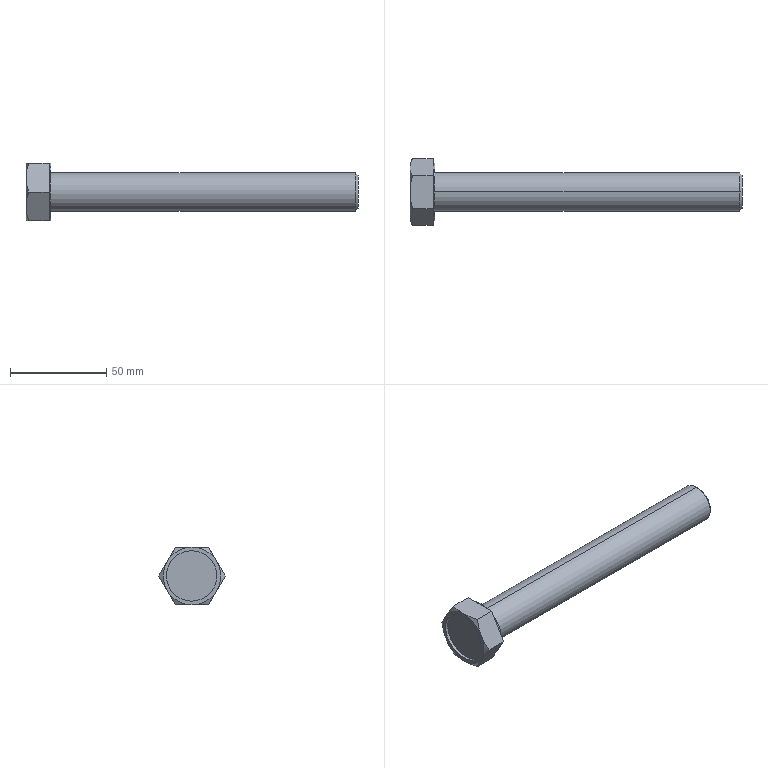Part | STEP file | formed hex screw_am_B18.2.3.2M - Formed hex screw, M20 x 2.5 x 160 --52WN | 1 solid | 30 faces | box 172.88 x 34.641 x 30 mm | volume 59289 mm3 | plane 16 | cone 8 | cylinder 6 | commonest cylinder face diameters 20 x2 26.25 x2 30 x2